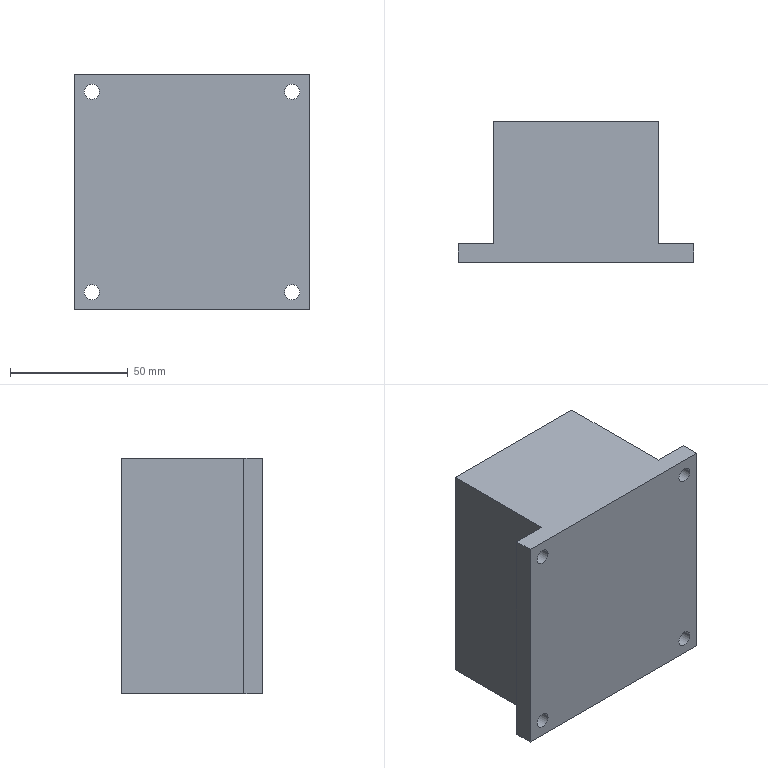Part | STEP file | X77a-01303 | 1 solid | 46 faces | box 100 x 60 x 100 mm | volume 441306 mm3 | cylinder 24 | plane 14 | cone 8 | commonest cylinder face diameters 5 x8 6 x8 6.5 x8
STEP:
#1=CARTESIAN_POINT('',(121.095,-100.053,3.986));
#2=VERTEX_POINT('',#1);
#3=CARTESIAN_POINT('',(121.095,-100.053,9.986));
#4=VERTEX_POINT('',#3);
#5=CARTESIAN_POINT('',(121.095,-100.053,6.986));
#6=DIRECTION('',(0.,1.,0.));
#7=DIRECTION('',(0.,0.,1.));
#8=AXIS2_PLACEMENT_3D('',#5,#6,#7);
#9=CIRCLE('',#8,3.);
#10=EDGE_CURVE('',#2,#4,#9,.T.);
#11=ORIENTED_EDGE('',*,*,#10,.F.);
#12=CARTESIAN_POINT('',(121.095,-88.053,3.986));
#13=VERTEX_POINT('',#12);
#14=CARTESIAN_POINT('',(121.095,-88.053,3.986));
#15=DIRECTION('',(0.,1.,0.));
#16=VECTOR('',#15,1000.);
#17=LINE('',#14,#16);
#18=EDGE_CURVE('',#2,#13,#17,.T.);
#19=ORIENTED_EDGE('',*,*,#18,.T.);
#20=CARTESIAN_POINT('',(121.095,-88.053,9.986));
#21=VERTEX_POINT('',#20);
#22=CARTESIAN_POINT('',(121.095,-88.053,6.986));
#23=DIRECTION('',(0.,1.,0.));
#24=DIRECTION('',(0.,0.,1.));
#25=AXIS2_PLACEMENT_3D('',#22,#23,#24);
#26=CIRCLE('',#25,3.);
#27=EDGE_CURVE('',#13,#21,#26,.T.);
#28=ORIENTED_EDGE('',*,*,#27,.T.);
#29=CARTESIAN_POINT('',(121.095,-88.053,9.986));
#30=DIRECTION('',(0.,1.,0.));
#31=VECTOR('',#30,1000.);
#32=LINE('',#29,#31);
#33=EDGE_CURVE('',#4,#21,#32,.T.);
#34=ORIENTED_EDGE('',*,*,#33,.F.);
#35=EDGE_LOOP('',(#11,#19,#28,#34));
#36=FACE_OUTER_BOUND('',#35,.T.);
#37=CARTESIAN_POINT('',(121.095,-88.053,6.986));
#38=DIRECTION('',(0.,1.,0.));
#39=DIRECTION('',(0.,0.,1.));
#40=AXIS2_PLACEMENT_3D('',#37,#38,#39);
#41=CYLINDRICAL_SURFACE('',#40,3.);
#42=ADVANCED_FACE('',(#36),#41,.F.);
#43=CARTESIAN_POINT('',(121.095,-103.053,4.486));
#44=VERTEX_POINT('',#43);
#45=CARTESIAN_POINT('',(121.095,-103.053,9.486));
#46=VERTEX_POINT('',#45);
#47=CARTESIAN_POINT('',(121.095,-103.053,6.986));
#48=DIRECTION('',(0.,1.,0.));
#49=DIRECTION('',(0.,0.,1.));
#50=AXIS2_PLACEMENT_3D('',#47,#48,#49);
#51=CIRCLE('',#50,2.5);
#52=EDGE_CURVE('',#44,#46,#51,.T.);
#53=ORIENTED_EDGE('',*,*,#52,.F.);
#54=CARTESIAN_POINT('',(121.095,-100.053,4.486));
#55=VERTEX_POINT('',#54);
#56=CARTESIAN_POINT('',(121.095,-88.053,4.486));
#57=DIRECTION('',(0.,1.,0.));
#58=VECTOR('',#57,1000.);
#59=LINE('',#56,#58);
#60=EDGE_CURVE('',#44,#55,#59,.T.);
#61=ORIENTED_EDGE('',*,*,#60,.T.);
#62=CARTESIAN_POINT('',(121.095,-100.053,9.486));
#63=VERTEX_POINT('',#62);
#64=CARTESIAN_POINT('',(121.095,-100.053,6.986));
#65=DIRECTION('',(0.,1.,0.));
#66=DIRECTION('',(0.,0.,1.));
#67=AXIS2_PLACEMENT_3D('',#64,#65,#66);
#68=CIRCLE('',#67,2.5);
#69=EDGE_CURVE('',#55,#63,#68,.T.);
#70=ORIENTED_EDGE('',*,*,#69,.T.);
#71=CARTESIAN_POINT('',(121.095,-88.053,9.486));
#72=DIRECTION('',(0.,1.,0.));
#73=VECTOR('',#72,1000.);
#74=LINE('',#71,#73);
#75=EDGE_CURVE('',#46,#63,#74,.T.);
#76=ORIENTED_EDGE('',*,*,#75,.F.);
#77=EDGE_LOOP('',(#53,#61,#70,#76));
#78=FACE_OUTER_BOUND('',#77,.T.);
#79=CARTESIAN_POINT('',(121.095,-88.053,6.986));
#80=DIRECTION('',(0.,1.,0.));
#81=DIRECTION('',(0.,0.,1.));
#82=AXIS2_PLACEMENT_3D('',#79,#80,#81);
#83=CYLINDRICAL_SURFACE('',#82,2.5);
#84=ADVANCED_FACE('',(#78),#83,.F.);
#85=CARTESIAN_POINT('',(121.095,-104.555,6.986));
#86=VERTEX_POINT('',#85);
#87=CARTESIAN_POINT('',(121.095,-103.053,9.486));
#88=DIRECTION('',(0.,0.515,0.8572));
#89=VECTOR('',#88,1000.);
#90=LINE('',#87,#89);
#91=EDGE_CURVE('',#86,#46,#90,.T.);
#92=ORIENTED_EDGE('',*,*,#91,.F.);
#93=CARTESIAN_POINT('',(121.095,-103.053,4.486));
#94=DIRECTION('',(0.,0.515,-0.8572));
#95=VECTOR('',#94,1000.);
#96=LINE('',#93,#95);
#97=EDGE_CURVE('',#86,#44,#96,.T.);
#98=ORIENTED_EDGE('',*,*,#97,.T.);
#99=ORIENTED_EDGE('',*,*,#52,.T.);
#100=EDGE_LOOP('',(#92,#98,#99));
#101=FACE_OUTER_BOUND('',#100,.T.);
#102=CARTESIAN_POINT('',(121.095,-103.053,6.986));
#103=DIRECTION('',(0.,1.,0.));
#104=DIRECTION('',(0.,0.,1.));
#105=AXIS2_PLACEMENT_3D('',#102,#103,#104);
#106=CONICAL_SURFACE('',#105,2.5,1.03);
#107=ADVANCED_FACE('',(#101),#106,.F.);
#108=CARTESIAN_POINT('',(176.095,-100.053,2.5));
#109=VERTEX_POINT('',#108);
#110=CARTESIAN_POINT('',(176.095,-100.053,8.5));
#111=VERTEX_POINT('',#110);
#112=CARTESIAN_POINT('',(176.095,-100.053,5.5));
#113=DIRECTION('',(0.,1.,0.));
#114=DIRECTION('',(0.,0.,1.));
#115=AXIS2_PLACEMENT_3D('',#112,#113,#114);
#116=CIRCLE('',#115,3.);
#117=EDGE_CURVE('',#109,#111,#116,.T.);
#118=ORIENTED_EDGE('',*,*,#117,.F.);
#119=CARTESIAN_POINT('',(176.095,-88.053,2.5));
#120=VERTEX_POINT('',#119);
#121=CARTESIAN_POINT('',(176.095,-88.053,2.5));
#122=DIRECTION('',(0.,1.,0.));
#123=VECTOR('',#122,1000.);
#124=LINE('',#121,#123);
#125=EDGE_CURVE('',#109,#120,#124,.T.);
#126=ORIENTED_EDGE('',*,*,#125,.T.);
#127=CARTESIAN_POINT('',(176.095,-88.053,8.5));
#128=VERTEX_POINT('',#127);
#129=CARTESIAN_POINT('',(176.095,-88.053,5.5));
#130=DIRECTION('',(0.,1.,0.));
#131=DIRECTION('',(0.,0.,1.));
#132=AXIS2_PLACEMENT_3D('',#129,#130,#131);
#133=CIRCLE('',#132,3.);
#134=EDGE_CURVE('',#120,#128,#133,.T.);
#135=ORIENTED_EDGE('',*,*,#134,.T.);
#136=CARTESIAN_POINT('',(176.095,-88.053,8.5));
#137=DIRECTION('',(0.,1.,0.));
#138=VECTOR('',#137,1000.);
#139=LINE('',#136,#138);
#140=EDGE_CURVE('',#111,#128,#139,.T.);
#141=ORIENTED_EDGE('',*,*,#140,.F.);
#142=EDGE_LOOP('',(#118,#126,#135,#141));
#143=FACE_OUTER_BOUND('',#142,.T.);
#144=CARTESIAN_POINT('',(176.095,-88.053,5.5));
#145=DIRECTION('',(0.,1.,0.));
#146=DIRECTION('',(0.,0.,1.));
#147=AXIS2_PLACEMENT_3D('',#144,#145,#146);
#148=CYLINDRICAL_SURFACE('',#147,3.);
#149=ADVANCED_FACE('',(#143),#148,.F.);
#150=CARTESIAN_POINT('',(176.095,-103.053,3.));
#151=VERTEX_POINT('',#150);
#152=CARTESIAN_POINT('',(176.095,-103.053,8.));
#153=VERTEX_POINT('',#152);
#154=CARTESIAN_POINT('',(176.095,-103.053,5.5));
#155=DIRECTION('',(0.,1.,0.));
#156=DIRECTION('',(0.,0.,1.));
#157=AXIS2_PLACEMENT_3D('',#154,#155,#156);
#158=CIRCLE('',#157,2.5);
#159=EDGE_CURVE('',#151,#153,#158,.T.);
#160=ORIENTED_EDGE('',*,*,#159,.F.);
#161=CARTESIAN_POINT('',(176.095,-100.053,3.));
#162=VERTEX_POINT('',#161);
#163=CARTESIAN_POINT('',(176.095,-88.053,3.));
#164=DIRECTION('',(0.,1.,0.));
#165=VECTOR('',#164,1000.);
#166=LINE('',#163,#165);
#167=EDGE_CURVE('',#151,#162,#166,.T.);
#168=ORIENTED_EDGE('',*,*,#167,.T.);
#169=CARTESIAN_POINT('',(176.095,-100.053,8.));
#170=VERTEX_POINT('',#169);
#171=CARTESIAN_POINT('',(176.095,-100.053,5.5));
#172=DIRECTION('',(0.,1.,0.));
#173=DIRECTION('',(0.,0.,1.));
#174=AXIS2_PLACEMENT_3D('',#171,#172,#173);
#175=CIRCLE('',#174,2.5);
#176=EDGE_CURVE('',#162,#170,#175,.T.);
#177=ORIENTED_EDGE('',*,*,#176,.T.);
#178=CARTESIAN_POINT('',(176.095,-88.053,8.));
#179=DIRECTION('',(0.,1.,0.));
#180=VECTOR('',#179,1000.);
#181=LINE('',#178,#180);
#182=EDGE_CURVE('',#153,#170,#181,.T.);
#183=ORIENTED_EDGE('',*,*,#182,.F.);
#184=EDGE_LOOP('',(#160,#168,#177,#183));
#185=FACE_OUTER_BOUND('',#184,.T.);
#186=CARTESIAN_POINT('',(176.095,-88.053,5.5));
#187=DIRECTION('',(0.,1.,0.));
#188=DIRECTION('',(0.,0.,1.));
#189=AXIS2_PLACEMENT_3D('',#186,#187,#188);
#190=CYLINDRICAL_SURFACE('',#189,2.5);
#191=ADVANCED_FACE('',(#185),#190,.F.);
#192=CARTESIAN_POINT('',(176.095,-104.555,5.5));
#193=VERTEX_POINT('',#192);
#194=CARTESIAN_POINT('',(176.095,-103.053,8.));
#195=DIRECTION('',(0.,0.515,0.8572));
#196=VECTOR('',#195,1000.);
#197=LINE('',#194,#196);
#198=EDGE_CURVE('',#193,#153,#197,.T.);
#199=ORIENTED_EDGE('',*,*,#198,.F.);
#200=CARTESIAN_POINT('',(176.095,-103.053,3.));
#201=DIRECTION('',(0.,0.515,-0.8572));
#202=VECTOR('',#201,1000.);
#203=LINE('',#200,#202);
#204=EDGE_CURVE('',#193,#151,#203,.T.);
#205=ORIENTED_EDGE('',*,*,#204,.T.);
#206=ORIENTED_EDGE('',*,*,#159,.T.);
#207=EDGE_LOOP('',(#199,#205,#206));
#208=FACE_OUTER_BOUND('',#207,.T.);
#209=CARTESIAN_POINT('',(176.095,-103.053,5.5));
#210=DIRECTION('',(0.,1.,0.));
#211=DIRECTION('',(0.,0.,1.));
#212=AXIS2_PLACEMENT_3D('',#209,#210,#211);
#213=CONICAL_SURFACE('',#212,2.5,1.03);
#214=ADVANCED_FACE('',(#208),#213,.F.);
#215=CARTESIAN_POINT('',(173.074,-100.053,91.5));
#216=VERTEX_POINT('',#215);
#217=CARTESIAN_POINT('',(173.074,-100.053,97.5));
#218=VERTEX_POINT('',#217);
#219=CARTESIAN_POINT('',(173.074,-100.053,94.5));
#220=DIRECTION('',(0.,1.,0.));
#221=DIRECTION('',(0.,0.,1.));
#222=AXIS2_PLACEMENT_3D('',#219,#220,#221);
#223=CIRCLE('',#222,3.);
#224=EDGE_CURVE('',#216,#218,#223,.T.);
#225=ORIENTED_EDGE('',*,*,#224,.F.);
#226=CARTESIAN_POINT('',(173.074,-88.053,91.5));
#227=VERTEX_POINT('',#226);
#228=CARTESIAN_POINT('',(173.074,-88.053,91.5));
#229=DIRECTION('',(0.,1.,0.));
#230=VECTOR('',#229,1000.);
#231=LINE('',#228,#230);
#232=EDGE_CURVE('',#216,#227,#231,.T.);
#233=ORIENTED_EDGE('',*,*,#232,.T.);
#234=CARTESIAN_POINT('',(173.074,-88.053,97.5));
#235=VERTEX_POINT('',#234);
#236=CARTESIAN_POINT('',(173.074,-88.053,94.5));
#237=DIRECTION('',(0.,1.,0.));
#238=DIRECTION('',(0.,0.,1.));
#239=AXIS2_PLACEMENT_3D('',#236,#237,#238);
#240=CIRCLE('',#239,3.);
#241=EDGE_CURVE('',#227,#235,#240,.T.);
#242=ORIENTED_EDGE('',*,*,#241,.T.);
#243=CARTESIAN_POINT('',(173.074,-88.053,97.5));
#244=DIRECTION('',(0.,1.,0.));
#245=VECTOR('',#244,1000.);
#246=LINE('',#243,#245);
#247=EDGE_CURVE('',#218,#235,#246,.T.);
#248=ORIENTED_EDGE('',*,*,#247,.F.);
#249=EDGE_LOOP('',(#225,#233,#242,#248));
#250=FACE_OUTER_BOUND('',#249,.T.);
#251=CARTESIAN_POINT('',(173.074,-88.053,94.5));
#252=DIRECTION('',(0.,1.,0.));
#253=DIRECTION('',(0.,0.,1.));
#254=AXIS2_PLACEMENT_3D('',#251,#252,#253);
#255=CYLINDRICAL_SURFACE('',#254,3.);
#256=ADVANCED_FACE('',(#250),#255,.F.);
#257=CARTESIAN_POINT('',(173.074,-103.053,92.));
#258=VERTEX_POINT('',#257);
#259=CARTESIAN_POINT('',(173.074,-103.053,97.));
#260=VERTEX_POINT('',#259);
#261=CARTESIAN_POINT('',(173.074,-103.053,94.5));
#262=DIRECTION('',(0.,1.,0.));
#263=DIRECTION('',(0.,0.,1.));
#264=AXIS2_PLACEMENT_3D('',#261,#262,#263);
#265=CIRCLE('',#264,2.5);
#266=EDGE_CURVE('',#258,#260,#265,.T.);
#267=ORIENTED_EDGE('',*,*,#266,.F.);
#268=CARTESIAN_POINT('',(173.074,-100.053,92.));
#269=VERTEX_POINT('',#268);
#270=CARTESIAN_POINT('',(173.074,-88.053,92.));
#271=DIRECTION('',(0.,1.,0.));
#272=VECTOR('',#271,1000.);
#273=LINE('',#270,#272);
#274=EDGE_CURVE('',#258,#269,#273,.T.);
#275=ORIENTED_EDGE('',*,*,#274,.T.);
#276=CARTESIAN_POINT('',(173.074,-100.053,97.));
#277=VERTEX_POINT('',#276);
#278=CARTESIAN_POINT('',(173.074,-100.053,94.5));
#279=DIRECTION('',(0.,1.,0.));
#280=DIRECTION('',(0.,0.,1.));
#281=AXIS2_PLACEMENT_3D('',#278,#279,#280);
#282=CIRCLE('',#281,2.5);
#283=EDGE_CURVE('',#269,#277,#282,.T.);
#284=ORIENTED_EDGE('',*,*,#283,.T.);
#285=CARTESIAN_POINT('',(173.074,-88.053,97.));
#286=DIRECTION('',(0.,1.,0.));
#287=VECTOR('',#286,1000.);
#288=LINE('',#285,#287);
#289=EDGE_CURVE('',#260,#277,#288,.T.);
#290=ORIENTED_EDGE('',*,*,#289,.F.);
#291=EDGE_LOOP('',(#267,#275,#284,#290));
#292=FACE_OUTER_BOUND('',#291,.T.);
#293=CARTESIAN_POINT('',(173.074,-88.053,94.5));
#294=DIRECTION('',(0.,1.,0.));
#295=DIRECTION('',(0.,0.,1.));
#296=AXIS2_PLACEMENT_3D('',#293,#294,#295);
#297=CYLINDRICAL_SURFACE('',#296,2.5);
#298=ADVANCED_FACE('',(#292),#297,.F.);
#299=CARTESIAN_POINT('',(173.074,-104.555,94.5));
#300=VERTEX_POINT('',#299);
#301=CARTESIAN_POINT('',(173.074,-103.053,97.));
#302=DIRECTION('',(0.,0.515,0.8572));
#303=VECTOR('',#302,1000.);
#304=LINE('',#301,#303);
#305=EDGE_CURVE('',#300,#260,#304,.T.);
#306=ORIENTED_EDGE('',*,*,#305,.F.);
#307=CARTESIAN_POINT('',(173.074,-103.053,92.));
#308=DIRECTION('',(0.,0.515,-0.8572));
#309=VECTOR('',#308,1000.);
#310=LINE('',#307,#309);
#311=EDGE_CURVE('',#300,#258,#310,.T.);
#312=ORIENTED_EDGE('',*,*,#311,.T.);
#313=ORIENTED_EDGE('',*,*,#266,.T.);
#314=EDGE_LOOP('',(#306,#312,#313));
#315=FACE_OUTER_BOUND('',#314,.T.);
#316=CARTESIAN_POINT('',(173.074,-103.053,94.5));
#317=DIRECTION('',(0.,1.,0.));
#318=DIRECTION('',(0.,0.,1.));
#319=AXIS2_PLACEMENT_3D('',#316,#317,#318);
#320=CONICAL_SURFACE('',#319,2.5,1.03);
#321=ADVANCED_FACE('',(#315),#320,.F.);
#322=CARTESIAN_POINT('',(121.095,-100.053,91.5));
#323=VERTEX_POINT('',#322);
#324=CARTESIAN_POINT('',(121.095,-100.053,97.5));
#325=VERTEX_POINT('',#324);
#326=CARTESIAN_POINT('',(121.095,-100.053,94.5));
#327=DIRECTION('',(0.,1.,0.));
#328=DIRECTION('',(0.,0.,1.));
#329=AXIS2_PLACEMENT_3D('',#326,#327,#328);
#330=CIRCLE('',#329,3.);
#331=EDGE_CURVE('',#323,#325,#330,.T.);
#332=ORIENTED_EDGE('',*,*,#331,.F.);
#333=CARTESIAN_POINT('',(121.095,-88.053,91.5));
#334=VERTEX_POINT('',#333);
#335=CARTESIAN_POINT('',(121.095,-88.053,91.5));
#336=DIRECTION('',(0.,1.,0.));
#337=VECTOR('',#336,1000.);
#338=LINE('',#335,#337);
#339=EDGE_CURVE('',#323,#334,#338,.T.);
#340=ORIENTED_EDGE('',*,*,#339,.T.);
#341=CARTESIAN_POINT('',(121.095,-88.053,97.5));
#342=VERTEX_POINT('',#341);
#343=CARTESIAN_POINT('',(121.095,-88.053,94.5));
#344=DIRECTION('',(0.,1.,0.));
#345=DIRECTION('',(0.,0.,1.));
#346=AXIS2_PLACEMENT_3D('',#343,#344,#345);
#347=CIRCLE('',#346,3.);
#348=EDGE_CURVE('',#334,#342,#347,.T.);
#349=ORIENTED_EDGE('',*,*,#348,.T.);
#350=CARTESIAN_POINT('',(121.095,-88.053,97.5));
#351=DIRECTION('',(0.,1.,0.));
#352=VECTOR('',#351,1000.);
#353=LINE('',#350,#352);
#354=EDGE_CURVE('',#325,#342,#353,.T.);
#355=ORIENTED_EDGE('',*,*,#354,.F.);
#356=EDGE_LOOP('',(#332,#340,#349,#355));
#357=FACE_OUTER_BOUND('',#356,.T.);
#358=CARTESIAN_POINT('',(121.095,-88.053,94.5));
#359=DIRECTION('',(0.,1.,0.));
#360=DIRECTION('',(0.,0.,1.));
#361=AXIS2_PLACEMENT_3D('',#358,#359,#360);
#362=CYLINDRICAL_SURFACE('',#361,3.);
#363=ADVANCED_FACE('',(#357),#362,.F.);
#364=CARTESIAN_POINT('',(121.095,-103.053,92.));
#365=VERTEX_POINT('',#364);
#366=CARTESIAN_POINT('',(121.095,-103.053,97.));
#367=VERTEX_POINT('',#366);
#368=CARTESIAN_POINT('',(121.095,-103.053,94.5));
#369=DIRECTION('',(0.,1.,0.));
#370=DIRECTION('',(0.,0.,1.));
#371=AXIS2_PLACEMENT_3D('',#368,#369,#370);
#372=CIRCLE('',#371,2.5);
#373=EDGE_CURVE('',#365,#367,#372,.T.);
#374=ORIENTED_EDGE('',*,*,#373,.F.);
#375=CARTESIAN_POINT('',(121.095,-100.053,92.));
#376=VERTEX_POINT('',#375);
#377=CARTESIAN_POINT('',(121.095,-88.053,92.));
#378=DIRECTION('',(0.,1.,0.));
#379=VECTOR('',#378,1000.);
#380=LINE('',#377,#379);
#381=EDGE_CURVE('',#365,#376,#380,.T.);
#382=ORIENTED_EDGE('',*,*,#381,.T.);
#383=CARTESIAN_POINT('',(121.095,-100.053,97.));
#384=VERTEX_POINT('',#383);
#385=CARTESIAN_POINT('',(121.095,-100.053,94.5));
#386=DIRECTION('',(0.,1.,0.));
#387=DIRECTION('',(0.,0.,1.));
#388=AXIS2_PLACEMENT_3D('',#385,#386,#387);
#389=CIRCLE('',#388,2.5);
#390=EDGE_CURVE('',#376,#384,#389,.T.);
#391=ORIENTED_EDGE('',*,*,#390,.T.);
#392=CARTESIAN_POINT('',(121.095,-88.053,97.));
#393=DIRECTION('',(0.,1.,0.));
#394=VECTOR('',#393,1000.);
#395=LINE('',#392,#394);
#396=EDGE_CURVE('',#367,#384,#395,.T.);
#397=ORIENTED_EDGE('',*,*,#396,.F.);
#398=EDGE_LOOP('',(#374,#382,#391,#397));
#399=FACE_OUTER_BOUND('',#398,.T.);
#400=CARTESIAN_POINT('',(121.095,-88.053,94.5));
#401=DIRECTION('',(0.,1.,0.));
#402=DIRECTION('',(0.,0.,1.));
#403=AXIS2_PLACEMENT_3D('',#400,#401,#402);
#404=CYLINDRICAL_SURFACE('',#403,2.5);
#405=ADVANCED_FACE('',(#399),#404,.F.);
#406=CARTESIAN_POINT('',(121.095,-104.555,94.5));
#407=VERTEX_POINT('',#406);
#408=CARTESIAN_POINT('',(121.095,-103.053,97.));
#409=DIRECTION('',(0.,0.515,0.8572));
#410=VECTOR('',#409,1000.);
#411=LINE('',#408,#410);
#412=EDGE_CURVE('',#407,#367,#411,.T.);
#413=ORIENTED_EDGE('',*,*,#412,.F.);
#414=CARTESIAN_POINT('',(121.095,-103.053,92.));
#415=DIRECTION('',(0.,0.515,-0.8572));
#416=VECTOR('',#415,1000.);
#417=LINE('',#414,#416);
#418=EDGE_CURVE('',#407,#365,#417,.T.);
#419=ORIENTED_EDGE('',*,*,#418,.T.);
#420=ORIENTED_EDGE('',*,*,#373,.T.);
#421=EDGE_LOOP('',(#413,#419,#420));
#422=FACE_OUTER_BOUND('',#421,.T.);
#423=CARTESIAN_POINT('',(121.095,-103.053,94.5));
#424=DIRECTION('',(0.,1.,0.));
#425=DIRECTION('',(0.,0.,1.));
#426=AXIS2_PLACEMENT_3D('',#423,#424,#425);
#427=CONICAL_SURFACE('',#426,2.5,1.03);
#428=ADVANCED_FACE('',(#422),#427,.F.);
#429=CARTESIAN_POINT('',(194.319,-148.053,92.5));
#430=VERTEX_POINT('',#429);
#431=CARTESIAN_POINT('',(187.819,-148.053,92.5));
#432=VERTEX_POINT('',#431);
#433=CARTESIAN_POINT('',(191.069,-148.053,92.5));
#434=DIRECTION('',(0.,1.,0.));
#435=DIRECTION('',(0.,0.,1.));
#436=AXIS2_PLACEMENT_3D('',#433,#434,#435);
#437=CIRCLE('',#436,3.25);
#438=EDGE_CURVE('',#430,#432,#437,.T.);
#439=ORIENTED_EDGE('',*,*,#438,.F.);
#440=CARTESIAN_POINT('',(194.319,-140.053,92.5));
#441=VERTEX_POINT('',#440);
#442=CARTESIAN_POINT('',(194.319,-150.053,92.5));
#443=DIRECTION('',(0.,1.,0.));
#444=VECTOR('',#443,1000.);
#445=LINE('',#442,#444);
#446=EDGE_CURVE('',#430,#441,#445,.T.);
#447=ORIENTED_EDGE('',*,*,#446,.T.);
#448=CARTESIAN_POINT('',(187.819,-140.053,92.5));
#449=VERTEX_POINT('',#448);
#450=CARTESIAN_POINT('',(191.069,-140.053,92.5));
#451=DIRECTION('',(0.,1.,0.));
#452=DIRECTION('',(1.,0.,0.));
#453=AXIS2_PLACEMENT_3D('',#450,#451,#452);
#454=CIRCLE('',#453,3.25);
#455=EDGE_CURVE('',#441,#449,#454,.T.);
#456=ORIENTED_EDGE('',*,*,#455,.T.);
#457=CARTESIAN_POINT('',(187.819,-150.053,92.5));
#458=DIRECTION('',(0.,1.,0.));
#459=VECTOR('',#458,1000.);
#460=LINE('',#457,#459);
#461=EDGE_CURVE('',#432,#449,#460,.T.);
#462=ORIENTED_EDGE('',*,*,#461,.F.);
#463=EDGE_LOOP('',(#439,#447,#456,#462));
#464=FACE_OUTER_BOUND('',#463,.T.);
#465=CARTESIAN_POINT('',(191.069,-150.053,92.5));
#466=DIRECTION('',(0.,1.,0.));
#467=DIRECTION('',(-1.,0.,0.));
#468=AXIS2_PLACEMENT_3D('',#465,#466,#467);
#469=CYLINDRICAL_SURFACE('',#468,3.25);
#470=ADVANCED_FACE('',(#464),#469,.F.);
#471=CARTESIAN_POINT('',(194.319,-148.053,7.5));
#472=VERTEX_POINT('',#471);
#473=CARTESIAN_POINT('',(187.819,-148.053,7.5));
#474=VERTEX_POINT('',#473);
#475=CARTESIAN_POINT('',(191.069,-148.053,7.5));
#476=DIRECTION('',(0.,1.,0.));
#477=DIRECTION('',(0.,0.,1.));
#478=AXIS2_PLACEMENT_3D('',#475,#476,#477);
#479=CIRCLE('',#478,3.25);
#480=EDGE_CURVE('',#472,#474,#479,.T.);
#481=ORIENTED_EDGE('',*,*,#480,.F.);
#482=CARTESIAN_POINT('',(194.319,-140.053,7.5));
#483=VERTEX_POINT('',#482);
#484=CARTESIAN_POINT('',(194.319,-150.053,7.5));
#485=DIRECTION('',(0.,1.,0.));
#486=VECTOR('',#485,1000.);
#487=LINE('',#484,#486);
#488=EDGE_CURVE('',#472,#483,#487,.T.);
#489=ORIENTED_EDGE('',*,*,#488,.T.);
#490=CARTESIAN_POINT('',(187.819,-140.053,7.5));
#491=VERTEX_POINT('',#490);
#492=CARTESIAN_POINT('',(191.069,-140.053,7.5));
#493=DIRECTION('',(0.,1.,0.));
#494=DIRECTION('',(1.,0.,0.));
#495=AXIS2_PLACEMENT_3D('',#492,#493,#494);
#496=CIRCLE('',#495,3.25);
#497=EDGE_CURVE('',#483,#491,#496,.T.);
#498=ORIENTED_EDGE('',*,*,#497,.T.);
#499=CARTESIAN_POINT('',(187.819,-150.053,7.5));
#500=DIRECTION('',(0.,1.,0.));
#501=VECTOR('',#500,1000.);
#502=LINE('',#499,#501);
#503=EDGE_CURVE('',#474,#491,#502,.T.);
#504=ORIENTED_EDGE('',*,*,#503,.F.);
#505=EDGE_LOOP('',(#481,#489,#498,#504));
#506=FACE_OUTER_BOUND('',#505,.T.);
#507=CARTESIAN_POINT('',(191.069,-150.053,7.5));
#508=DIRECTION('',(0.,1.,0.));
#509=DIRECTION('',(-1.,0.,0.));
#510=AXIS2_PLACEMENT_3D('',#507,#508,#509);
#511=CYLINDRICAL_SURFACE('',#510,3.25);
#512=ADVANCED_FACE('',(#506),#511,.F.);
#513=CARTESIAN_POINT('',(109.37,-148.053,92.5));
#514=VERTEX_POINT('',#513);
#515=CARTESIAN_POINT('',(102.87,-148.053,92.5));
#516=VERTEX_POINT('',#515);
#517=CARTESIAN_POINT('',(106.12,-148.053,92.5));
#518=DIRECTION('',(0.,1.,0.));
#519=DIRECTION('',(0.,0.,1.));
#520=AXIS2_PLACEMENT_3D('',#517,#518,#519);
#521=CIRCLE('',#520,3.25);
#522=EDGE_CURVE('',#514,#516,#521,.T.);
#523=ORIENTED_EDGE('',*,*,#522,.F.);
#524=CARTESIAN_POINT('',(109.37,-140.053,92.5));
#525=VERTEX_POINT('',#524);
#526=CARTESIAN_POINT('',(109.37,-150.053,92.5));
#527=DIRECTION('',(0.,1.,0.));
#528=VECTOR('',#527,1000.);
#529=LINE('',#526,#528);
#530=EDGE_CURVE('',#514,#525,#529,.T.);
#531=ORIENTED_EDGE('',*,*,#530,.T.);
#532=CARTESIAN_POINT('',(102.87,-140.053,92.5));
#533=VERTEX_POINT('',#532);
#534=CARTESIAN_POINT('',(106.12,-140.053,92.5));
#535=DIRECTION('',(0.,1.,0.));
#536=DIRECTION('',(-1.,0.,0.));
#537=AXIS2_PLACEMENT_3D('',#534,#535,#536);
#538=CIRCLE('',#537,3.25);
#539=EDGE_CURVE('',#525,#533,#538,.T.);
#540=ORIENTED_EDGE('',*,*,#539,.T.);
#541=CARTESIAN_POINT('',(102.87,-150.053,92.5));
#542=DIRECTION('',(0.,1.,0.));
#543=VECTOR('',#542,1000.);
#544=LINE('',#541,#543);
#545=EDGE_CURVE('',#516,#533,#544,.T.);
#546=ORIENTED_EDGE('',*,*,#545,.F.);
#547=EDGE_LOOP('',(#523,#531,#540,#546));
#548=FACE_OUTER_BOUND('',#547,.T.);
#549=CARTESIAN_POINT('',(106.12,-150.053,92.5));
#550=DIRECTION('',(0.,1.,0.));
#551=DIRECTION('',(-1.,0.,0.));
#552=AXIS2_PLACEMENT_3D('',#549,#550,#551);
#553=CYLINDRICAL_SURFACE('',#552,3.25);
#554=ADVANCED_FACE('',(#548),#553,.F.);
#555=CARTESIAN_POINT('',(109.37,-148.053,7.5));
#556=VERTEX_POINT('',#555);
#557=CARTESIAN_POINT('',(102.87,-148.053,7.5));
#558=VERTEX_POINT('',#557);
#559=CARTESIAN_POINT('',(106.12,-148.053,7.5));
#560=DIRECTION('',(0.,1.,0.));
#561=DIRECTION('',(0.,0.,1.));
#562=AXIS2_PLACEMENT_3D('',#559,#560,#561);
#563=CIRCLE('',#562,3.25);
#564=EDGE_CURVE('',#556,#558,#563,.T.);
#565=ORIENTED_EDGE('',*,*,#564,.F.);
#566=CARTESIAN_POINT('',(109.37,-140.053,7.5));
#567=VERTEX_POINT('',#566);
#568=CARTESIAN_POINT('',(109.37,-150.053,7.5));
#569=DIRECTION('',(0.,1.,0.));
#570=VECTOR('',#569,1000.);
#571=LINE('',#568,#570);
#572=EDGE_CURVE('',#556,#567,#571,.T.);
#573=ORIENTED_EDGE('',*,*,#572,.T.);
#574=CARTESIAN_POINT('',(102.87,-140.053,7.5));
#575=VERTEX_POINT('',#574);
#576=CARTESIAN_POINT('',(106.12,-140.053,7.5));
#577=DIRECTION('',(0.,1.,0.));
#578=DIRECTION('',(-1.,0.,0.));
#579=AXIS2_PLACEMENT_3D('',#576,#577,#578);
#580=CIRCLE('',#579,3.25);
#581=EDGE_CURVE('',#567,#575,#580,.T.);
#582=ORIENTED_EDGE('',*,*,#581,.T.);
#583=CARTESIAN_POINT('',(102.87,-150.053,7.5));
#584=DIRECTION('',(0.,1.,0.));
#585=VECTOR('',#584,1000.);
#586=LINE('',#583,#585);
#587=EDGE_CURVE('',#558,#575,#586,.T.);
#588=ORIENTED_EDGE('',*,*,#587,.F.);
#589=EDGE_LOOP('',(#565,#573,#582,#588));
#590=FACE_OUTER_BOUND('',#589,.T.);
#591=CARTESIAN_POINT('',(106.12,-150.053,7.5));
#592=DIRECTION('',(0.,1.,0.));
#593=DIRECTION('',(-1.,0.,0.));
#594=AXIS2_PLACEMENT_3D('',#591,#592,#593);
#595=CYLINDRICAL_SURFACE('',#594,3.25);
#596=ADVANCED_FACE('',(#590),#595,.F.);
#597=CARTESIAN_POINT('',(121.095,-88.053,6.986));
#598=DIRECTION('',(0.,1.,0.));
#599=DIRECTION('',(0.,0.,1.));
#600=AXIS2_PLACEMENT_3D('',#597,#598,#599);
#601=CIRCLE('',#600,3.);
#602=EDGE_CURVE('',#21,#13,#601,.T.);
#603=ORIENTED_EDGE('',*,*,#602,.F.);
#604=ORIENTED_EDGE('',*,*,#27,.F.);
#605=EDGE_LOOP('',(#603,#604));
#606=FACE_BOUND('',#605,.T.);
#607=CARTESIAN_POINT('',(176.095,-88.053,5.5));
#608=DIRECTION('',(0.,1.,0.));
#609=DIRECTION('',(0.,0.,1.));
#610=AXIS2_PLACEMENT_3D('',#607,#608,#609);
#611=CIRCLE('',#610,3.);
#612=EDGE_CURVE('',#128,#120,#611,.T.);
#613=ORIENTED_EDGE('',*,*,#612,.F.);
#614=ORIENTED_EDGE('',*,*,#134,.F.);
#615=EDGE_LOOP('',(#613,#614));
#616=FACE_BOUND('',#615,.T.);
#617=CARTESIAN_POINT('',(173.074,-88.053,94.5));
#618=DIRECTION('',(0.,1.,0.));
#619=DIRECTION('',(0.,0.,1.));
#620=AXIS2_PLACEMENT_3D('',#617,#618,#619);
#621=CIRCLE('',#620,3.);
#622=EDGE_CURVE('',#235,#227,#621,.T.);
#623=ORIENTED_EDGE('',*,*,#622,.F.);
#624=ORIENTED_EDGE('',*,*,#241,.F.);
#625=EDGE_LOOP('',(#623,#624));
#626=FACE_BOUND('',#625,.T.);
#627=CARTESIAN_POINT('',(121.095,-88.053,94.5));
#628=DIRECTION('',(0.,1.,0.));
#629=DIRECTION('',(0.,0.,1.));
#630=AXIS2_PLACEMENT_3D('',#627,#628,#629);
#631=CIRCLE('',#630,3.);
#632=EDGE_CURVE('',#342,#334,#631,.T.);
#633=ORIENTED_EDGE('',*,*,#632,.F.);
#634=ORIENTED_EDGE('',*,*,#348,.F.);
#635=EDGE_LOOP('',(#633,#634));
#636=FACE_BOUND('',#635,.T.);
#637=CARTESIAN_POINT('',(183.595,-88.053,0.));
#638=VERTEX_POINT('',#637);
#639=CARTESIAN_POINT('',(113.595,-88.053,0.));
#640=VERTEX_POINT('',#639);
#641=CARTESIAN_POINT('',(183.595,-88.053,0.));
#642=DIRECTION('',(-1.,0.,0.));
#643=VECTOR('',#642,1000.);
#644=LINE('',#641,#643);
#645=EDGE_CURVE('',#638,#640,#644,.T.);
#646=ORIENTED_EDGE('',*,*,#645,.T.);
#647=CARTESIAN_POINT('',(113.595,-88.053,100.));
#648=VERTEX_POINT('',#647);
#649=CARTESIAN_POINT('',(113.595,-88.053,100.));
#650=DIRECTION('',(0.,0.,-1.));
#651=VECTOR('',#650,1000.);
#652=LINE('',#649,#651);
#653=EDGE_CURVE('',#648,#640,#652,.T.);
#654=ORIENTED_EDGE('',*,*,#653,.F.);
#655=CARTESIAN_POINT('',(183.595,-88.053,100.));
#656=VERTEX_POINT('',#655);
#657=CARTESIAN_POINT('',(183.595,-88.053,100.));
#658=DIRECTION('',(-1.,0.,0.));
#659=VECTOR('',#658,1000.);
#660=LINE('',#657,#659);
#661=EDGE_CURVE('',#656,#648,#660,.T.);
#662=ORIENTED_EDGE('',*,*,#661,.F.);
#663=CARTESIAN_POINT('',(183.595,-88.053,100.));
#664=DIRECTION('',(0.,0.,-1.));
#665=VECTOR('',#664,1000.);
#666=LINE('',#663,#665);
#667=EDGE_CURVE('',#656,#638,#666,.T.);
#668=ORIENTED_EDGE('',*,*,#667,.T.);
#669=EDGE_LOOP('',(#646,#654,#662,#668));
#670=FACE_OUTER_BOUND('',#669,.T.);
#671=CARTESIAN_POINT('',(183.595,-88.053,100.));
#672=DIRECTION('',(0.,-1.,0.));
#673=DIRECTION('',(1.,0.,0.));
#674=AXIS2_PLACEMENT_3D('',#671,#672,#673);
#675=PLANE('',#674);
#676=ADVANCED_FACE('',(#606,#616,#626,#636,#670),#675,.F.);
#677=CARTESIAN_POINT('',(113.595,-140.053,0.));
#678=VERTEX_POINT('',#677);
#679=CARTESIAN_POINT('',(113.595,-88.053,0.));
#680=DIRECTION('',(0.,-1.,0.));
#681=VECTOR('',#680,1000.);
#682=LINE('',#679,#681);
#683=EDGE_CURVE('',#640,#678,#682,.T.);
#684=ORIENTED_EDGE('',*,*,#683,.T.);
#685=CARTESIAN_POINT('',(113.595,-140.053,100.));
#686=VERTEX_POINT('',#685);
#687=CARTESIAN_POINT('',(113.595,-140.053,100.));
#688=DIRECTION('',(0.,0.,-1.));
#689=VECTOR('',#688,1000.);
#690=LINE('',#687,#689);
#691=EDGE_CURVE('',#686,#678,#690,.T.);
#692=ORIENTED_EDGE('',*,*,#691,.F.);
#693=CARTESIAN_POINT('',(113.595,-88.053,100.));
#694=DIRECTION('',(0.,-1.,0.));
#695=VECTOR('',#694,1000.);
#696=LINE('',#693,#695);
#697=EDGE_CURVE('',#648,#686,#696,.T.);
#698=ORIENTED_EDGE('',*,*,#697,.F.);
#699=ORIENTED_EDGE('',*,*,#653,.T.);
#700=EDGE_LOOP('',(#684,#692,#698,#699));
#701=FACE_OUTER_BOUND('',#700,.T.);
#702=CARTESIAN_POINT('',(113.595,-88.053,100.));
#703=DIRECTION('',(1.,0.,0.));
#704=DIRECTION('',(0.,0.,-1.));
#705=AXIS2_PLACEMENT_3D('',#702,#703,#704);
#706=PLANE('',#705);
#707=ADVANCED_FACE('',(#701),#706,.F.);
#708=CARTESIAN_POINT('',(106.12,-140.053,92.5));
#709=DIRECTION('',(0.,1.,0.));
#710=DIRECTION('',(-1.,0.,0.));
#711=AXIS2_PLACEMENT_3D('',#708,#709,#710);
#712=CIRCLE('',#711,3.25);
#713=EDGE_CURVE('',#533,#525,#712,.T.);
#714=ORIENTED_EDGE('',*,*,#713,.F.);
#715=ORIENTED_EDGE('',*,*,#539,.F.);
#716=EDGE_LOOP('',(#714,#715));
#717=FACE_BOUND('',#716,.T.);
#718=CARTESIAN_POINT('',(106.12,-140.053,7.5));
#719=DIRECTION('',(0.,1.,0.));
#720=DIRECTION('',(-1.,0.,0.));
#721=AXIS2_PLACEMENT_3D('',#718,#719,#720);
#722=CIRCLE('',#721,3.25);
#723=EDGE_CURVE('',#575,#567,#722,.T.);
#724=ORIENTED_EDGE('',*,*,#723,.F.);
#725=ORIENTED_EDGE('',*,*,#581,.F.);
#726=EDGE_LOOP('',(#724,#725));
#727=FACE_BOUND('',#726,.T.);
#728=CARTESIAN_POINT('',(98.595,-140.053,0.));
#729=VERTEX_POINT('',#728);
#730=CARTESIAN_POINT('',(113.595,-140.053,0.));
#731=DIRECTION('',(-1.,0.,0.));
#732=VECTOR('',#731,1000.);
#733=LINE('',#730,#732);
#734=EDGE_CURVE('',#678,#729,#733,.T.);
#735=ORIENTED_EDGE('',*,*,#734,.T.);
#736=CARTESIAN_POINT('',(98.595,-140.053,100.));
#737=VERTEX_POINT('',#736);
#738=CARTESIAN_POINT('',(98.595,-140.053,100.));
#739=DIRECTION('',(0.,0.,-1.));
#740=VECTOR('',#739,1000.);
#741=LINE('',#738,#740);
#742=EDGE_CURVE('',#737,#729,#741,.T.);
#743=ORIENTED_EDGE('',*,*,#742,.F.);
#744=CARTESIAN_POINT('',(113.595,-140.053,100.));
#745=DIRECTION('',(-1.,0.,0.));
#746=VECTOR('',#745,1000.);
#747=LINE('',#744,#746);
#748=EDGE_CURVE('',#686,#737,#747,.T.);
#749=ORIENTED_EDGE('',*,*,#748,.F.);
#750=ORIENTED_EDGE('',*,*,#691,.T.);
#751=EDGE_LOOP('',(#735,#743,#749,#750));
#752=FACE_OUTER_BOUND('',#751,.T.);
#753=CARTESIAN_POINT('',(113.595,-140.053,100.));
#754=DIRECTION('',(0.,-1.,0.));
#755=DIRECTION('',(0.,0.,-1.));
#756=AXIS2_PLACEMENT_3D('',#753,#754,#755);
#757=PLANE('',#756);
#758=ADVANCED_FACE('',(#717,#727,#752),#757,.F.);
#759=CARTESIAN_POINT('',(98.595,-148.053,0.));
#760=VERTEX_POINT('',#759);
#761=CARTESIAN_POINT('',(98.595,-140.053,0.));
#762=DIRECTION('',(0.,-1.,0.));
#763=VECTOR('',#762,1000.);
#764=LINE('',#761,#763);
#765=EDGE_CURVE('',#729,#760,#764,.T.);
#766=ORIENTED_EDGE('',*,*,#765,.T.);
#767=CARTESIAN_POINT('',(98.595,-148.053,100.));
#768=VERTEX_POINT('',#767);
#769=CARTESIAN_POINT('',(98.595,-148.053,100.));
#770=DIRECTION('',(0.,0.,-1.));
#771=VECTOR('',#770,1000.);
#772=LINE('',#769,#771);
#773=EDGE_CURVE('',#768,#760,#772,.T.);
#774=ORIENTED_EDGE('',*,*,#773,.F.);
#775=CARTESIAN_POINT('',(98.595,-140.053,100.));
#776=DIRECTION('',(0.,-1.,0.));
#777=VECTOR('',#776,1000.);
#778=LINE('',#775,#777);
#779=EDGE_CURVE('',#737,#768,#778,.T.);
#780=ORIENTED_EDGE('',*,*,#779,.F.);
#781=ORIENTED_EDGE('',*,*,#742,.T.);
#782=EDGE_LOOP('',(#766,#774,#780,#781));
#783=FACE_OUTER_BOUND('',#782,.T.);
#784=CARTESIAN_POINT('',(98.595,-140.053,100.));
#785=DIRECTION('',(1.,0.,0.));
#786=DIRECTION('',(0.,0.,-1.));
#787=AXIS2_PLACEMENT_3D('',#784,#785,#786);
#788=PLANE('',#787);
#789=ADVANCED_FACE('',(#783),#788,.F.);
#790=CARTESIAN_POINT('',(191.069,-148.053,92.5));
#791=DIRECTION('',(0.,1.,0.));
#792=DIRECTION('',(0.,0.,1.));
#793=AXIS2_PLACEMENT_3D('',#790,#791,#792);
#794=CIRCLE('',#793,3.25);
#795=EDGE_CURVE('',#432,#430,#794,.T.);
#796=ORIENTED_EDGE('',*,*,#795,.T.);
#797=ORIENTED_EDGE('',*,*,#438,.T.);
#798=EDGE_LOOP('',(#796,#797));
#799=FACE_BOUND('',#798,.T.);
#800=CARTESIAN_POINT('',(191.069,-148.053,7.5));
#801=DIRECTION('',(0.,1.,0.));
#802=DIRECTION('',(0.,0.,1.));
#803=AXIS2_PLACEMENT_3D('',#800,#801,#802);
#804=CIRCLE('',#803,3.25);
#805=EDGE_CURVE('',#474,#472,#804,.T.);
#806=ORIENTED_EDGE('',*,*,#805,.T.);
#807=ORIENTED_EDGE('',*,*,#480,.T.);
#808=EDGE_LOOP('',(#806,#807));
#809=FACE_BOUND('',#808,.T.);
#810=CARTESIAN_POINT('',(106.12,-148.053,92.5));
#811=DIRECTION('',(0.,1.,0.));
#812=DIRECTION('',(0.,0.,1.));
#813=AXIS2_PLACEMENT_3D('',#810,#811,#812);
#814=CIRCLE('',#813,3.25);
#815=EDGE_CURVE('',#516,#514,#814,.T.);
#816=ORIENTED_EDGE('',*,*,#815,.T.);
#817=ORIENTED_EDGE('',*,*,#522,.T.);
#818=EDGE_LOOP('',(#816,#817));
#819=FACE_BOUND('',#818,.T.);
#820=CARTESIAN_POINT('',(106.12,-148.053,7.5));
#821=DIRECTION('',(0.,1.,0.));
#822=DIRECTION('',(0.,0.,1.));
#823=AXIS2_PLACEMENT_3D('',#820,#821,#822);
#824=CIRCLE('',#823,3.25);
#825=EDGE_CURVE('',#558,#556,#824,.T.);
#826=ORIENTED_EDGE('',*,*,#825,.T.);
#827=ORIENTED_EDGE('',*,*,#564,.T.);
#828=EDGE_LOOP('',(#826,#827));
#829=FACE_BOUND('',#828,.T.);
#830=CARTESIAN_POINT('',(198.595,-148.053,0.));
#831=VERTEX_POINT('',#830);
#832=CARTESIAN_POINT('',(98.595,-148.053,0.));
#833=DIRECTION('',(1.,0.,0.));
#834=VECTOR('',#833,1000.);
#835=LINE('',#832,#834);
#836=EDGE_CURVE('',#760,#831,#835,.T.);
#837=ORIENTED_EDGE('',*,*,#836,.T.);
#838=CARTESIAN_POINT('',(198.595,-148.053,100.));
#839=VERTEX_POINT('',#838);
#840=CARTESIAN_POINT('',(198.595,-148.053,100.));
#841=DIRECTION('',(0.,0.,-1.));
#842=VECTOR('',#841,1000.);
#843=LINE('',#840,#842);
#844=EDGE_CURVE('',#839,#831,#843,.T.);
#845=ORIENTED_EDGE('',*,*,#844,.F.);
#846=CARTESIAN_POINT('',(98.595,-148.053,100.));
#847=DIRECTION('',(1.,0.,0.));
#848=VECTOR('',#847,1000.);
#849=LINE('',#846,#848);
#850=EDGE_CURVE('',#768,#839,#849,.T.);
#851=ORIENTED_EDGE('',*,*,#850,.F.);
#852=ORIENTED_EDGE('',*,*,#773,.T.);
#853=EDGE_LOOP('',(#837,#845,#851,#852));
#854=FACE_OUTER_BOUND('',#853,.T.);
#855=CARTESIAN_POINT('',(98.595,-148.053,100.));
#856=DIRECTION('',(0.,1.,0.));
#857=DIRECTION('',(0.,0.,1.));
#858=AXIS2_PLACEMENT_3D('',#855,#856,#857);
#859=PLANE('',#858);
#860=ADVANCED_FACE('',(#799,#809,#819,#829,#854),#859,.F.);
#861=CARTESIAN_POINT('',(198.595,-140.053,0.));
#862=VERTEX_POINT('',#861);
#863=CARTESIAN_POINT('',(198.595,-148.053,0.));
#864=DIRECTION('',(0.,1.,0.));
#865=VECTOR('',#864,1000.);
#866=LINE('',#863,#865);
#867=EDGE_CURVE('',#831,#862,#866,.T.);
#868=ORIENTED_EDGE('',*,*,#867,.T.);
#869=CARTESIAN_POINT('',(198.595,-140.053,100.));
#870=VERTEX_POINT('',#869);
#871=CARTESIAN_POINT('',(198.595,-140.053,100.));
#872=DIRECTION('',(0.,0.,-1.));
#873=VECTOR('',#872,1000.);
#874=LINE('',#871,#873);
#875=EDGE_CURVE('',#870,#862,#874,.T.);
#876=ORIENTED_EDGE('',*,*,#875,.F.);
#877=CARTESIAN_POINT('',(198.595,-148.053,100.));
#878=DIRECTION('',(0.,1.,0.));
#879=VECTOR('',#878,1000.);
#880=LINE('',#877,#879);
#881=EDGE_CURVE('',#839,#870,#880,.T.);
#882=ORIENTED_EDGE('',*,*,#881,.F.);
#883=ORIENTED_EDGE('',*,*,#844,.T.);
#884=EDGE_LOOP('',(#868,#876,#882,#883));
#885=FACE_OUTER_BOUND('',#884,.T.);
#886=CARTESIAN_POINT('',(198.595,-148.053,100.));
#887=DIRECTION('',(-1.,0.,0.));
#888=DIRECTION('',(0.,0.,1.));
#889=AXIS2_PLACEMENT_3D('',#886,#887,#888);
#890=PLANE('',#889);
#891=ADVANCED_FACE('',(#885),#890,.F.);
#892=CARTESIAN_POINT('',(191.069,-140.053,92.5));
#893=DIRECTION('',(0.,1.,0.));
#894=DIRECTION('',(1.,0.,0.));
#895=AXIS2_PLACEMENT_3D('',#892,#893,#894);
#896=CIRCLE('',#895,3.25);
#897=EDGE_CURVE('',#449,#441,#896,.T.);
#898=ORIENTED_EDGE('',*,*,#897,.F.);
#899=ORIENTED_EDGE('',*,*,#455,.F.);
#900=EDGE_LOOP('',(#898,#899));
#901=FACE_BOUND('',#900,.T.);
#902=CARTESIAN_POINT('',(191.069,-140.053,7.5));
#903=DIRECTION('',(0.,1.,0.));
#904=DIRECTION('',(1.,0.,0.));
#905=AXIS2_PLACEMENT_3D('',#902,#903,#904);
#906=CIRCLE('',#905,3.25);
#907=EDGE_CURVE('',#491,#483,#906,.T.);
#908=ORIENTED_EDGE('',*,*,#907,.F.);
#909=ORIENTED_EDGE('',*,*,#497,.F.);
#910=EDGE_LOOP('',(#908,#909));
#911=FACE_BOUND('',#910,.T.);
#912=CARTESIAN_POINT('',(183.595,-140.053,0.));
#913=VERTEX_POINT('',#912);
#914=CARTESIAN_POINT('',(198.595,-140.053,0.));
#915=DIRECTION('',(-1.,0.,0.));
#916=VECTOR('',#915,1000.);
#917=LINE('',#914,#916);
#918=EDGE_CURVE('',#862,#913,#917,.T.);
#919=ORIENTED_EDGE('',*,*,#918,.T.);
#920=CARTESIAN_POINT('',(183.595,-140.053,100.));
#921=VERTEX_POINT('',#920);
#922=CARTESIAN_POINT('',(183.595,-140.053,100.));
#923=DIRECTION('',(0.,0.,-1.));
#924=VECTOR('',#923,1000.);
#925=LINE('',#922,#924);
#926=EDGE_CURVE('',#921,#913,#925,.T.);
#927=ORIENTED_EDGE('',*,*,#926,.F.);
#928=CARTESIAN_POINT('',(198.595,-140.053,100.));
#929=DIRECTION('',(-1.,0.,0.));
#930=VECTOR('',#929,1000.);
#931=LINE('',#928,#930);
#932=EDGE_CURVE('',#870,#921,#931,.T.);
#933=ORIENTED_EDGE('',*,*,#932,.F.);
#934=ORIENTED_EDGE('',*,*,#875,.T.);
#935=EDGE_LOOP('',(#919,#927,#933,#934));
#936=FACE_OUTER_BOUND('',#935,.T.);
#937=CARTESIAN_POINT('',(198.595,-140.053,100.));
#938=DIRECTION('',(0.,-1.,0.));
#939=DIRECTION('',(0.,0.,-1.));
#940=AXIS2_PLACEMENT_3D('',#937,#938,#939);
#941=PLANE('',#940);
#942=ADVANCED_FACE('',(#901,#911,#936),#941,.F.);
#943=CARTESIAN_POINT('',(183.595,-140.053,0.));
#944=DIRECTION('',(0.,1.,0.));
#945=VECTOR('',#944,1000.);
#946=LINE('',#943,#945);
#947=EDGE_CURVE('',#913,#638,#946,.T.);
#948=ORIENTED_EDGE('',*,*,#947,.T.);
#949=ORIENTED_EDGE('',*,*,#667,.F.);
#950=CARTESIAN_POINT('',(183.595,-140.053,100.));
#951=DIRECTION('',(0.,1.,0.));
#952=VECTOR('',#951,1000.);
#953=LINE('',#950,#952);
#954=EDGE_CURVE('',#921,#656,#953,.T.);
#955=ORIENTED_EDGE('',*,*,#954,.F.);
#956=ORIENTED_EDGE('',*,*,#926,.T.);
#957=EDGE_LOOP('',(#948,#949,#955,#956));
#958=FACE_OUTER_BOUND('',#957,.T.);
#959=CARTESIAN_POINT('',(183.595,-140.053,100.));
#960=DIRECTION('',(-1.,0.,0.));
#961=DIRECTION('',(0.,0.,1.));
#962=AXIS2_PLACEMENT_3D('',#959,#960,#961);
#963=PLANE('',#962);
#964=ADVANCED_FACE('',(#958),#963,.F.);
#965=ORIENTED_EDGE('',*,*,#661,.T.);
#966=ORIENTED_EDGE('',*,*,#697,.T.);
#967=ORIENTED_EDGE('',*,*,#748,.T.);
#968=ORIENTED_EDGE('',*,*,#779,.T.);
#969=ORIENTED_EDGE('',*,*,#850,.T.);
#970=ORIENTED_EDGE('',*,*,#881,.T.);
#971=ORIENTED_EDGE('',*,*,#932,.T.);
#972=ORIENTED_EDGE('',*,*,#954,.T.);
#973=EDGE_LOOP('',(#965,#966,#967,#968,#969,#970,#971,#972));
#974=FACE_OUTER_BOUND('',#973,.T.);
#975=CARTESIAN_POINT('',(113.595,-88.053,100.));
#976=DIRECTION('',(0.,0.,1.));
#977=DIRECTION('',(1.,0.,0.));
#978=AXIS2_PLACEMENT_3D('',#975,#976,#977);
#979=PLANE('',#978);
#980=ADVANCED_FACE('',(#974),#979,.T.);
#981=ORIENTED_EDGE('',*,*,#645,.F.);
#982=ORIENTED_EDGE('',*,*,#947,.F.);
#983=ORIENTED_EDGE('',*,*,#918,.F.);
#984=ORIENTED_EDGE('',*,*,#867,.F.);
#985=ORIENTED_EDGE('',*,*,#836,.F.);
#986=ORIENTED_EDGE('',*,*,#765,.F.);
#987=ORIENTED_EDGE('',*,*,#734,.F.);
#988=ORIENTED_EDGE('',*,*,#683,.F.);
#989=EDGE_LOOP('',(#981,#982,#983,#984,#985,#986,#987,#988));
#990=FACE_OUTER_BOUND('',#989,.T.);
#991=CARTESIAN_POINT('',(113.595,-88.053,0.));
#992=DIRECTION('',(0.,0.,1.));
#993=DIRECTION('',(1.,0.,0.));
#994=AXIS2_PLACEMENT_3D('',#991,#992,#993);
#995=PLANE('',#994);
#996=ADVANCED_FACE('',(#990),#995,.F.);
#997=ORIENTED_EDGE('',*,*,#572,.F.);
#998=ORIENTED_EDGE('',*,*,#825,.F.);
#999=ORIENTED_EDGE('',*,*,#587,.T.);
#1000=ORIENTED_EDGE('',*,*,#723,.T.);
#1001=EDGE_LOOP('',(#997,#998,#999,#1000));
#1002=FACE_OUTER_BOUND('',#1001,.T.);
#1003=CARTESIAN_POINT('',(106.12,-150.053,7.5));
#1004=DIRECTION('',(0.,1.,0.));
#1005=DIRECTION('',(-1.,0.,0.));
#1006=AXIS2_PLACEMENT_3D('',#1003,#1004,#1005);
#1007=CYLINDRICAL_SURFACE('',#1006,3.25);
#1008=ADVANCED_FACE('',(#1002),#1007,.F.);
#1009=ORIENTED_EDGE('',*,*,#530,.F.);
#1010=ORIENTED_EDGE('',*,*,#815,.F.);
#1011=ORIENTED_EDGE('',*,*,#545,.T.);
#1012=ORIENTED_EDGE('',*,*,#713,.T.);
#1013=EDGE_LOOP('',(#1009,#1010,#1011,#1012));
#1014=FACE_OUTER_BOUND('',#1013,.T.);
#1015=CARTESIAN_POINT('',(106.12,-150.053,92.5));
#1016=DIRECTION('',(0.,1.,0.));
#1017=DIRECTION('',(-1.,0.,0.));
#1018=AXIS2_PLACEMENT_3D('',#1015,#1016,#1017);
#1019=CYLINDRICAL_SURFACE('',#1018,3.25);
#1020=ADVANCED_FACE('',(#1014),#1019,.F.);
#1021=ORIENTED_EDGE('',*,*,#488,.F.);
#1022=ORIENTED_EDGE('',*,*,#805,.F.);
#1023=ORIENTED_EDGE('',*,*,#503,.T.);
#1024=ORIENTED_EDGE('',*,*,#907,.T.);
#1025=EDGE_LOOP('',(#1021,#1022,#1023,#1024));
#1026=FACE_OUTER_BOUND('',#1025,.T.);
#1027=CARTESIAN_POINT('',(191.069,-150.053,7.5));
#1028=DIRECTION('',(0.,1.,0.));
#1029=DIRECTION('',(-1.,0.,0.));
#1030=AXIS2_PLACEMENT_3D('',#1027,#1028,#1029);
#1031=CYLINDRICAL_SURFACE('',#1030,3.25);
#1032=ADVANCED_FACE('',(#1026),#1031,.F.);
#1033=ORIENTED_EDGE('',*,*,#446,.F.);
#1034=ORIENTED_EDGE('',*,*,#795,.F.);
#1035=ORIENTED_EDGE('',*,*,#461,.T.);
#1036=ORIENTED_EDGE('',*,*,#897,.T.);
#1037=EDGE_LOOP('',(#1033,#1034,#1035,#1036));
#1038=FACE_OUTER_BOUND('',#1037,.T.);
#1039=CARTESIAN_POINT('',(191.069,-150.053,92.5));
#1040=DIRECTION('',(0.,1.,0.));
#1041=DIRECTION('',(-1.,0.,0.));
#1042=AXIS2_PLACEMENT_3D('',#1039,#1040,#1041);
#1043=CYLINDRICAL_SURFACE('',#1042,3.25);
#1044=ADVANCED_FACE('',(#1038),#1043,.F.);
#1045=ORIENTED_EDGE('',*,*,#418,.F.);
#1046=ORIENTED_EDGE('',*,*,#412,.T.);
#1047=CARTESIAN_POINT('',(121.095,-103.053,94.5));
#1048=DIRECTION('',(0.,1.,0.));
#1049=DIRECTION('',(0.,0.,1.));
#1050=AXIS2_PLACEMENT_3D('',#1047,#1048,#1049);
#1051=CIRCLE('',#1050,2.5);
#1052=EDGE_CURVE('',#367,#365,#1051,.T.);
#1053=ORIENTED_EDGE('',*,*,#1052,.T.);
#1054=EDGE_LOOP('',(#1045,#1046,#1053));
#1055=FACE_OUTER_BOUND('',#1054,.T.);
#1056=CARTESIAN_POINT('',(121.095,-103.053,94.5));
#1057=DIRECTION('',(0.,1.,0.));
#1058=DIRECTION('',(0.,0.,1.));
#1059=AXIS2_PLACEMENT_3D('',#1056,#1057,#1058);
#1060=CONICAL_SURFACE('',#1059,2.5,1.03);
#1061=ADVANCED_FACE('',(#1055),#1060,.F.);
#1062=ORIENTED_EDGE('',*,*,#381,.F.);
#1063=ORIENTED_EDGE('',*,*,#1052,.F.);
#1064=ORIENTED_EDGE('',*,*,#396,.T.);
#1065=CARTESIAN_POINT('',(121.095,-100.053,94.5));
#1066=DIRECTION('',(0.,1.,0.));
#1067=DIRECTION('',(0.,0.,1.));
#1068=AXIS2_PLACEMENT_3D('',#1065,#1066,#1067);
#1069=CIRCLE('',#1068,2.5);
#1070=EDGE_CURVE('',#384,#376,#1069,.T.);
#1071=ORIENTED_EDGE('',*,*,#1070,.T.);
#1072=EDGE_LOOP('',(#1062,#1063,#1064,#1071));
#1073=FACE_OUTER_BOUND('',#1072,.T.);
#1074=CARTESIAN_POINT('',(121.095,-88.053,94.5));
#1075=DIRECTION('',(0.,1.,0.));
#1076=DIRECTION('',(0.,0.,1.));
#1077=AXIS2_PLACEMENT_3D('',#1074,#1075,#1076);
#1078=CYLINDRICAL_SURFACE('',#1077,2.5);
#1079=ADVANCED_FACE('',(#1073),#1078,.F.);
#1080=ORIENTED_EDGE('',*,*,#1070,.F.);
#1081=ORIENTED_EDGE('',*,*,#390,.F.);
#1082=EDGE_LOOP('',(#1080,#1081));
#1083=FACE_BOUND('',#1082,.T.);
#1084=CARTESIAN_POINT('',(121.095,-100.053,94.5));
#1085=DIRECTION('',(0.,1.,0.));
#1086=DIRECTION('',(0.,0.,1.));
#1087=AXIS2_PLACEMENT_3D('',#1084,#1085,#1086);
#1088=CIRCLE('',#1087,3.);
#1089=EDGE_CURVE('',#325,#323,#1088,.T.);
#1090=ORIENTED_EDGE('',*,*,#1089,.T.);
#1091=ORIENTED_EDGE('',*,*,#331,.T.);
#1092=EDGE_LOOP('',(#1090,#1091));
#1093=FACE_OUTER_BOUND('',#1092,.T.);
#1094=CARTESIAN_POINT('',(123.595,-100.053,94.5));
#1095=DIRECTION('',(0.,-1.,0.));
#1096=DIRECTION('',(0.,0.,-1.));
#1097=AXIS2_PLACEMENT_3D('',#1094,#1095,#1096);
#1098=PLANE('',#1097);
#1099=ADVANCED_FACE('',(#1083,#1093),#1098,.F.);
#1100=ORIENTED_EDGE('',*,*,#339,.F.);
#1101=ORIENTED_EDGE('',*,*,#1089,.F.);
#1102=ORIENTED_EDGE('',*,*,#354,.T.);
#1103=ORIENTED_EDGE('',*,*,#632,.T.);
#1104=EDGE_LOOP('',(#1100,#1101,#1102,#1103));
#1105=FACE_OUTER_BOUND('',#1104,.T.);
#1106=CARTESIAN_POINT('',(121.095,-88.053,94.5));
#1107=DIRECTION('',(0.,1.,0.));
#1108=DIRECTION('',(0.,0.,1.));
#1109=AXIS2_PLACEMENT_3D('',#1106,#1107,#1108);
#1110=CYLINDRICAL_SURFACE('',#1109,3.);
#1111=ADVANCED_FACE('',(#1105),#1110,.F.);
#1112=ORIENTED_EDGE('',*,*,#311,.F.);
#1113=ORIENTED_EDGE('',*,*,#305,.T.);
#1114=CARTESIAN_POINT('',(173.074,-103.053,94.5));
#1115=DIRECTION('',(0.,1.,0.));
#1116=DIRECTION('',(0.,0.,1.));
#1117=AXIS2_PLACEMENT_3D('',#1114,#1115,#1116);
#1118=CIRCLE('',#1117,2.5);
#1119=EDGE_CURVE('',#260,#258,#1118,.T.);
#1120=ORIENTED_EDGE('',*,*,#1119,.T.);
#1121=EDGE_LOOP('',(#1112,#1113,#1120));
#1122=FACE_OUTER_BOUND('',#1121,.T.);
#1123=CARTESIAN_POINT('',(173.074,-103.053,94.5));
#1124=DIRECTION('',(0.,1.,0.));
#1125=DIRECTION('',(0.,0.,1.));
#1126=AXIS2_PLACEMENT_3D('',#1123,#1124,#1125);
#1127=CONICAL_SURFACE('',#1126,2.5,1.03);
#1128=ADVANCED_FACE('',(#1122),#1127,.F.);
#1129=ORIENTED_EDGE('',*,*,#274,.F.);
#1130=ORIENTED_EDGE('',*,*,#1119,.F.);
#1131=ORIENTED_EDGE('',*,*,#289,.T.);
#1132=CARTESIAN_POINT('',(173.074,-100.053,94.5));
#1133=DIRECTION('',(0.,1.,0.));
#1134=DIRECTION('',(0.,0.,1.));
#1135=AXIS2_PLACEMENT_3D('',#1132,#1133,#1134);
#1136=CIRCLE('',#1135,2.5);
#1137=EDGE_CURVE('',#277,#269,#1136,.T.);
#1138=ORIENTED_EDGE('',*,*,#1137,.T.);
#1139=EDGE_LOOP('',(#1129,#1130,#1131,#1138));
#1140=FACE_OUTER_BOUND('',#1139,.T.);
#1141=CARTESIAN_POINT('',(173.074,-88.053,94.5));
#1142=DIRECTION('',(0.,1.,0.));
#1143=DIRECTION('',(0.,0.,1.));
#1144=AXIS2_PLACEMENT_3D('',#1141,#1142,#1143);
#1145=CYLINDRICAL_SURFACE('',#1144,2.5);
#1146=ADVANCED_FACE('',(#1140),#1145,.F.);
#1147=ORIENTED_EDGE('',*,*,#1137,.F.);
#1148=ORIENTED_EDGE('',*,*,#283,.F.);
#1149=EDGE_LOOP('',(#1147,#1148));
#1150=FACE_BOUND('',#1149,.T.);
#1151=CARTESIAN_POINT('',(173.074,-100.053,94.5));
#1152=DIRECTION('',(0.,1.,0.));
#1153=DIRECTION('',(0.,0.,1.));
#1154=AXIS2_PLACEMENT_3D('',#1151,#1152,#1153);
#1155=CIRCLE('',#1154,3.);
#1156=EDGE_CURVE('',#218,#216,#1155,.T.);
#1157=ORIENTED_EDGE('',*,*,#1156,.T.);
#1158=ORIENTED_EDGE('',*,*,#224,.T.);
#1159=EDGE_LOOP('',(#1157,#1158));
#1160=FACE_OUTER_BOUND('',#1159,.T.);
#1161=CARTESIAN_POINT('',(175.574,-100.053,94.5));
#1162=DIRECTION('',(0.,-1.,0.));
#1163=DIRECTION('',(0.,0.,-1.));
#1164=AXIS2_PLACEMENT_3D('',#1161,#1162,#1163);
#1165=PLANE('',#1164);
#1166=ADVANCED_FACE('',(#1150,#1160),#1165,.F.);
#1167=ORIENTED_EDGE('',*,*,#232,.F.);
#1168=ORIENTED_EDGE('',*,*,#1156,.F.);
#1169=ORIENTED_EDGE('',*,*,#247,.T.);
#1170=ORIENTED_EDGE('',*,*,#622,.T.);
#1171=EDGE_LOOP('',(#1167,#1168,#1169,#1170));
#1172=FACE_OUTER_BOUND('',#1171,.T.);
#1173=CARTESIAN_POINT('',(173.074,-88.053,94.5));
#1174=DIRECTION('',(0.,1.,0.));
#1175=DIRECTION('',(0.,0.,1.));
#1176=AXIS2_PLACEMENT_3D('',#1173,#1174,#1175);
#1177=CYLINDRICAL_SURFACE('',#1176,3.);
#1178=ADVANCED_FACE('',(#1172),#1177,.F.);
#1179=ORIENTED_EDGE('',*,*,#204,.F.);
#1180=ORIENTED_EDGE('',*,*,#198,.T.);
#1181=CARTESIAN_POINT('',(176.095,-103.053,5.5));
#1182=DIRECTION('',(0.,1.,0.));
#1183=DIRECTION('',(0.,0.,1.));
#1184=AXIS2_PLACEMENT_3D('',#1181,#1182,#1183);
#1185=CIRCLE('',#1184,2.5);
#1186=EDGE_CURVE('',#153,#151,#1185,.T.);
#1187=ORIENTED_EDGE('',*,*,#1186,.T.);
#1188=EDGE_LOOP('',(#1179,#1180,#1187));
#1189=FACE_OUTER_BOUND('',#1188,.T.);
#1190=CARTESIAN_POINT('',(176.095,-103.053,5.5));
#1191=DIRECTION('',(0.,1.,0.));
#1192=DIRECTION('',(0.,0.,1.));
#1193=AXIS2_PLACEMENT_3D('',#1190,#1191,#1192);
#1194=CONICAL_SURFACE('',#1193,2.5,1.03);
#1195=ADVANCED_FACE('',(#1189),#1194,.F.);
#1196=ORIENTED_EDGE('',*,*,#167,.F.);
#1197=ORIENTED_EDGE('',*,*,#1186,.F.);
#1198=ORIENTED_EDGE('',*,*,#182,.T.);
#1199=CARTESIAN_POINT('',(176.095,-100.053,5.5));
#1200=DIRECTION('',(0.,1.,0.));
#1201=DIRECTION('',(0.,0.,1.));
#1202=AXIS2_PLACEMENT_3D('',#1199,#1200,#1201);
#1203=CIRCLE('',#1202,2.5);
#1204=EDGE_CURVE('',#170,#162,#1203,.T.);
#1205=ORIENTED_EDGE('',*,*,#1204,.T.);
#1206=EDGE_LOOP('',(#1196,#1197,#1198,#1205));
#1207=FACE_OUTER_BOUND('',#1206,.T.);
#1208=CARTESIAN_POINT('',(176.095,-88.053,5.5));
#1209=DIRECTION('',(0.,1.,0.));
#1210=DIRECTION('',(0.,0.,1.));
#1211=AXIS2_PLACEMENT_3D('',#1208,#1209,#1210);
#1212=CYLINDRICAL_SURFACE('',#1211,2.5);
#1213=ADVANCED_FACE('',(#1207),#1212,.F.);
#1214=ORIENTED_EDGE('',*,*,#1204,.F.);
#1215=ORIENTED_EDGE('',*,*,#176,.F.);
#1216=EDGE_LOOP('',(#1214,#1215));
#1217=FACE_BOUND('',#1216,.T.);
#1218=CARTESIAN_POINT('',(176.095,-100.053,5.5));
#1219=DIRECTION('',(0.,1.,0.));
#1220=DIRECTION('',(0.,0.,1.));
#1221=AXIS2_PLACEMENT_3D('',#1218,#1219,#1220);
#1222=CIRCLE('',#1221,3.);
#1223=EDGE_CURVE('',#111,#109,#1222,.T.);
#1224=ORIENTED_EDGE('',*,*,#1223,.T.);
#1225=ORIENTED_EDGE('',*,*,#117,.T.);
#1226=EDGE_LOOP('',(#1224,#1225));
#1227=FACE_OUTER_BOUND('',#1226,.T.);
#1228=CARTESIAN_POINT('',(178.595,-100.053,5.5));
#1229=DIRECTION('',(0.,-1.,0.));
#1230=DIRECTION('',(0.,0.,-1.));
#1231=AXIS2_PLACEMENT_3D('',#1228,#1229,#1230);
#1232=PLANE('',#1231);
#1233=ADVANCED_FACE('',(#1217,#1227),#1232,.F.);
#1234=ORIENTED_EDGE('',*,*,#125,.F.);
#1235=ORIENTED_EDGE('',*,*,#1223,.F.);
#1236=ORIENTED_EDGE('',*,*,#140,.T.);
#1237=ORIENTED_EDGE('',*,*,#612,.T.);
#1238=EDGE_LOOP('',(#1234,#1235,#1236,#1237));
#1239=FACE_OUTER_BOUND('',#1238,.T.);
#1240=CARTESIAN_POINT('',(176.095,-88.053,5.5));
#1241=DIRECTION('',(0.,1.,0.));
#1242=DIRECTION('',(0.,0.,1.));
#1243=AXIS2_PLACEMENT_3D('',#1240,#1241,#1242);
#1244=CYLINDRICAL_SURFACE('',#1243,3.);
#1245=ADVANCED_FACE('',(#1239),#1244,.F.);
#1246=ORIENTED_EDGE('',*,*,#97,.F.);
#1247=ORIENTED_EDGE('',*,*,#91,.T.);
#1248=CARTESIAN_POINT('',(121.095,-103.053,6.986));
#1249=DIRECTION('',(0.,1.,0.));
#1250=DIRECTION('',(0.,0.,1.));
#1251=AXIS2_PLACEMENT_3D('',#1248,#1249,#1250);
#1252=CIRCLE('',#1251,2.5);
#1253=EDGE_CURVE('',#46,#44,#1252,.T.);
#1254=ORIENTED_EDGE('',*,*,#1253,.T.);
#1255=EDGE_LOOP('',(#1246,#1247,#1254));
#1256=FACE_OUTER_BOUND('',#1255,.T.);
#1257=CARTESIAN_POINT('',(121.095,-103.053,6.986));
#1258=DIRECTION('',(0.,1.,0.));
#1259=DIRECTION('',(0.,0.,1.));
#1260=AXIS2_PLACEMENT_3D('',#1257,#1258,#1259);
#1261=CONICAL_SURFACE('',#1260,2.5,1.03);
#1262=ADVANCED_FACE('',(#1256),#1261,.F.);
#1263=ORIENTED_EDGE('',*,*,#60,.F.);
#1264=ORIENTED_EDGE('',*,*,#1253,.F.);
#1265=ORIENTED_EDGE('',*,*,#75,.T.);
#1266=CARTESIAN_POINT('',(121.095,-100.053,6.986));
#1267=DIRECTION('',(0.,1.,0.));
#1268=DIRECTION('',(0.,0.,1.));
#1269=AXIS2_PLACEMENT_3D('',#1266,#1267,#1268);
#1270=CIRCLE('',#1269,2.5);
#1271=EDGE_CURVE('',#63,#55,#1270,.T.);
#1272=ORIENTED_EDGE('',*,*,#1271,.T.);
#1273=EDGE_LOOP('',(#1263,#1264,#1265,#1272));
#1274=FACE_OUTER_BOUND('',#1273,.T.);
#1275=CARTESIAN_POINT('',(121.095,-88.053,6.986));
#1276=DIRECTION('',(0.,1.,0.));
#1277=DIRECTION('',(0.,0.,1.));
#1278=AXIS2_PLACEMENT_3D('',#1275,#1276,#1277);
#1279=CYLINDRICAL_SURFACE('',#1278,2.5);
#1280=ADVANCED_FACE('',(#1274),#1279,.F.);
#1281=ORIENTED_EDGE('',*,*,#1271,.F.);
#1282=ORIENTED_EDGE('',*,*,#69,.F.);
#1283=EDGE_LOOP('',(#1281,#1282));
#1284=FACE_BOUND('',#1283,.T.);
#1285=CARTESIAN_POINT('',(121.095,-100.053,6.986));
#1286=DIRECTION('',(0.,1.,0.));
#1287=DIRECTION('',(0.,0.,1.));
#1288=AXIS2_PLACEMENT_3D('',#1285,#1286,#1287);
#1289=CIRCLE('',#1288,3.);
#1290=EDGE_CURVE('',#4,#2,#1289,.T.);
#1291=ORIENTED_EDGE('',*,*,#1290,.T.);
#1292=ORIENTED_EDGE('',*,*,#10,.T.);
#1293=EDGE_LOOP('',(#1291,#1292));
#1294=FACE_OUTER_BOUND('',#1293,.T.);
#1295=CARTESIAN_POINT('',(123.595,-100.053,6.986));
#1296=DIRECTION('',(0.,-1.,0.));
#1297=DIRECTION('',(0.,0.,-1.));
#1298=AXIS2_PLACEMENT_3D('',#1295,#1296,#1297);
#1299=PLANE('',#1298);
#1300=ADVANCED_FACE('',(#1284,#1294),#1299,.F.);
#1301=ORIENTED_EDGE('',*,*,#18,.F.);
#1302=ORIENTED_EDGE('',*,*,#1290,.F.);
#1303=ORIENTED_EDGE('',*,*,#33,.T.);
#1304=ORIENTED_EDGE('',*,*,#602,.T.);
#1305=EDGE_LOOP('',(#1301,#1302,#1303,#1304));
#1306=FACE_OUTER_BOUND('',#1305,.T.);
#1307=CARTESIAN_POINT('',(121.095,-88.053,6.986));
#1308=DIRECTION('',(0.,1.,0.));
#1309=DIRECTION('',(0.,0.,1.));
#1310=AXIS2_PLACEMENT_3D('',#1307,#1308,#1309);
#1311=CYLINDRICAL_SURFACE('',#1310,3.);
#1312=ADVANCED_FACE('',(#1306),#1311,.F.);
#1313=CLOSED_SHELL('',(#42,#84,#107,#149,#191,#214,#256,#298,#321,#363,#405,#428,#470,#512,#554,#596,#676,#707,#758,#789,#860,#891,#942,#964,#980,#996,#1008,#1020,#1032,#1044,#1061,#1079,#1099,#1111,#1128,#1146,#1166,#1178,#1195,#1213,#1233,#1245,#1262,#1280,#1300,#1312));
#1314=MANIFOLD_SOLID_BREP('',#1313);
#1315=CARTESIAN_POINT('',(0.,0.,0.));
#1316=DIRECTION('',(0.,0.,1.));
#1317=DIRECTION('',(1.,0.,0.));
#1318=AXIS2_PLACEMENT_3D('',#1315,#1316,#1317);
#1319=(LENGTH_UNIT()NAMED_UNIT(*)SI_UNIT(.MILLI.,.METRE.));
#1320=UNCERTAINTY_MEASURE_WITH_UNIT(LENGTH_MEASURE(0.00001),#1319,'','');
#1321=(NAMED_UNIT(*)PLANE_ANGLE_UNIT()SI_UNIT($,.RADIAN.));
#1322=(NAMED_UNIT(*)SI_UNIT($,.STERADIAN.)SOLID_ANGLE_UNIT());
#1323=(GEOMETRIC_REPRESENTATION_CONTEXT(3)GLOBAL_UNCERTAINTY_ASSIGNED_CONTEXT((#1320))GLOBAL_UNIT_ASSIGNED_CONTEXT((#1319,#1321,#1322))REPRESENTATION_CONTEXT('',''));
#1324=ADVANCED_BREP_SHAPE_REPRESENTATION('',(#1314,#1318),#1323);